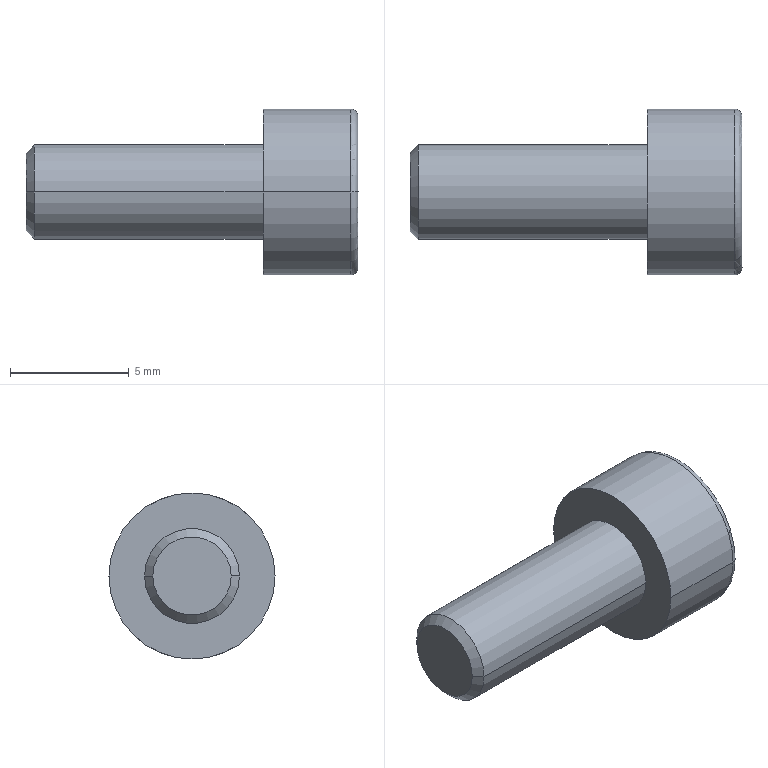Part | STEP file | 4-20.sldasm-Part-7 | 1 solid | 18 faces | box 14 x 7 x 7 mm | volume 262.874 mm3 | plane 10 | cylinder 4 | cone 2 | torus 2 | commonest cylinder face diameters 4 x2 7 x2
STEP:
#1=CARTESIAN_POINT('',(255.,438.35,193.));
#2=VERTEX_POINT('',#1);
#3=CARTESIAN_POINT('',(255.,441.651,193.));
#4=VERTEX_POINT('',#3);
#5=CARTESIAN_POINT('',(255.,440.,193.));
#6=DIRECTION('',(1.,0.000000295,0.));
#7=DIRECTION('',(-0.000000295,1.,-0.000000295));
#8=AXIS2_PLACEMENT_3D('',#5,#6,#7);
#9=CIRCLE('',#8,1.65);
#10=EDGE_CURVE('',#2,#4,#9,.T.);
#11=ORIENTED_EDGE('',*,*,#10,.T.);
#12=CARTESIAN_POINT('',(255.349,442.,193.));
#13=VERTEX_POINT('',#12);
#14=CARTESIAN_POINT('',(255.349,442.,193.));
#15=DIRECTION('',(0.7071,0.7071,-0.000000209));
#16=VECTOR('',#15,1000.);
#17=LINE('',#14,#16);
#18=EDGE_CURVE('',#4,#13,#17,.T.);
#19=ORIENTED_EDGE('',*,*,#18,.T.);
#20=CARTESIAN_POINT('',(255.349,438.,193.));
#21=VERTEX_POINT('',#20);
#22=CARTESIAN_POINT('',(255.349,440.,193.));
#23=DIRECTION('',(1.,0.000000295,0.));
#24=DIRECTION('',(-0.000000295,1.,-0.000000295));
#25=AXIS2_PLACEMENT_3D('',#22,#23,#24);
#26=CIRCLE('',#25,2.);
#27=EDGE_CURVE('',#21,#13,#26,.T.);
#28=ORIENTED_EDGE('',*,*,#27,.F.);
#29=CARTESIAN_POINT('',(255.349,438.,193.));
#30=DIRECTION('',(0.7071,-0.7071,0.000000209));
#31=VECTOR('',#30,1000.);
#32=LINE('',#29,#31);
#33=EDGE_CURVE('',#2,#21,#32,.T.);
#34=ORIENTED_EDGE('',*,*,#33,.F.);
#35=EDGE_LOOP('',(#11,#19,#28,#34));
#36=FACE_OUTER_BOUND('',#35,.T.);
#37=CARTESIAN_POINT('',(255.349,440.,193.));
#38=DIRECTION('',(1.,0.000000295,0.));
#39=DIRECTION('',(0.000000295,-1.,0.000000295));
#40=AXIS2_PLACEMENT_3D('',#37,#38,#39);
#41=CONICAL_SURFACE('',#40,2.,0.7854);
#42=ADVANCED_FACE('',(#36),#41,.T.);
#43=ORIENTED_EDGE('',*,*,#27,.T.);
#44=CARTESIAN_POINT('',(265.,442.,193.));
#45=VERTEX_POINT('',#44);
#46=CARTESIAN_POINT('',(270.675,442.,193.));
#47=DIRECTION('',(1.,0.000000295,0.));
#48=VECTOR('',#47,1000.);
#49=LINE('',#46,#48);
#50=EDGE_CURVE('',#13,#45,#49,.T.);
#51=ORIENTED_EDGE('',*,*,#50,.T.);
#52=CARTESIAN_POINT('',(265.,438.,193.));
#53=VERTEX_POINT('',#52);
#54=CARTESIAN_POINT('',(265.,440.,193.));
#55=DIRECTION('',(1.,0.000000295,0.));
#56=DIRECTION('',(-0.000000295,1.,-0.000000295));
#57=AXIS2_PLACEMENT_3D('',#54,#55,#56);
#58=CIRCLE('',#57,2.);
#59=EDGE_CURVE('',#53,#45,#58,.T.);
#60=ORIENTED_EDGE('',*,*,#59,.F.);
#61=CARTESIAN_POINT('',(270.675,438.,193.));
#62=DIRECTION('',(1.,0.000000295,0.));
#63=VECTOR('',#62,1000.);
#64=LINE('',#61,#63);
#65=EDGE_CURVE('',#21,#53,#64,.T.);
#66=ORIENTED_EDGE('',*,*,#65,.F.);
#67=EDGE_LOOP('',(#43,#51,#60,#66));
#68=FACE_OUTER_BOUND('',#67,.T.);
#69=CARTESIAN_POINT('',(270.675,440.,193.));
#70=DIRECTION('',(1.,0.000000295,0.));
#71=DIRECTION('',(0.000000295,-1.,0.000000295));
#72=AXIS2_PLACEMENT_3D('',#69,#70,#71);
#73=CYLINDRICAL_SURFACE('',#72,2.);
#74=ADVANCED_FACE('',(#68),#73,.T.);
#75=CARTESIAN_POINT('',(265.,436.5,193.));
#76=VERTEX_POINT('',#75);
#77=CARTESIAN_POINT('',(265.,443.5,193.));
#78=VERTEX_POINT('',#77);
#79=CARTESIAN_POINT('',(265.,440.,193.));
#80=DIRECTION('',(1.,0.000000295,0.));
#81=DIRECTION('',(-0.000000295,1.,-0.000000295));
#82=AXIS2_PLACEMENT_3D('',#79,#80,#81);
#83=CIRCLE('',#82,3.5);
#84=EDGE_CURVE('',#76,#78,#83,.T.);
#85=ORIENTED_EDGE('',*,*,#84,.T.);
#86=CARTESIAN_POINT('',(268.7,443.5,193.));
#87=VERTEX_POINT('',#86);
#88=CARTESIAN_POINT('',(270.675,443.5,193.));
#89=DIRECTION('',(1.,0.000000295,0.));
#90=VECTOR('',#89,1000.);
#91=LINE('',#88,#90);
#92=EDGE_CURVE('',#78,#87,#91,.T.);
#93=ORIENTED_EDGE('',*,*,#92,.T.);
#94=CARTESIAN_POINT('',(268.7,436.5,193.));
#95=VERTEX_POINT('',#94);
#96=CARTESIAN_POINT('',(268.7,440.,193.));
#97=DIRECTION('',(1.,0.000000295,0.));
#98=DIRECTION('',(-0.000000295,1.,-0.000000295));
#99=AXIS2_PLACEMENT_3D('',#96,#97,#98);
#100=CIRCLE('',#99,3.5);
#101=EDGE_CURVE('',#95,#87,#100,.T.);
#102=ORIENTED_EDGE('',*,*,#101,.F.);
#103=CARTESIAN_POINT('',(270.675,436.5,193.));
#104=DIRECTION('',(1.,0.000000295,0.));
#105=VECTOR('',#104,1000.);
#106=LINE('',#103,#105);
#107=EDGE_CURVE('',#76,#95,#106,.T.);
#108=ORIENTED_EDGE('',*,*,#107,.F.);
#109=EDGE_LOOP('',(#85,#93,#102,#108));
#110=FACE_OUTER_BOUND('',#109,.T.);
#111=CARTESIAN_POINT('',(270.675,440.,193.));
#112=DIRECTION('',(1.,0.000000295,0.));
#113=DIRECTION('',(0.000000295,-1.,0.000000295));
#114=AXIS2_PLACEMENT_3D('',#111,#112,#113);
#115=CYLINDRICAL_SURFACE('',#114,3.5);
#116=ADVANCED_FACE('',(#110),#115,.T.);
#117=ORIENTED_EDGE('',*,*,#101,.T.);
#118=CARTESIAN_POINT('',(269.,443.2,193.));
#119=VERTEX_POINT('',#118);
#120=CARTESIAN_POINT('',(268.7,443.2,193.));
#121=DIRECTION('',(0.,-0.000000295,-1.));
#122=DIRECTION('',(0.,1.,-0.000000295));
#123=AXIS2_PLACEMENT_3D('',#120,#121,#122);
#124=CIRCLE('',#123,0.3);
#125=EDGE_CURVE('',#87,#119,#124,.T.);
#126=ORIENTED_EDGE('',*,*,#125,.T.);
#127=CARTESIAN_POINT('',(269.,436.8,193.));
#128=VERTEX_POINT('',#127);
#129=CARTESIAN_POINT('',(269.,440.,193.));
#130=DIRECTION('',(1.,0.000000295,0.));
#131=DIRECTION('',(-0.000000295,1.,-0.000000295));
#132=AXIS2_PLACEMENT_3D('',#129,#130,#131);
#133=CIRCLE('',#132,3.2);
#134=EDGE_CURVE('',#128,#119,#133,.T.);
#135=ORIENTED_EDGE('',*,*,#134,.F.);
#136=CARTESIAN_POINT('',(268.7,436.8,193.));
#137=DIRECTION('',(0.,0.000000295,1.));
#138=DIRECTION('',(0.,-1.,0.000000295));
#139=AXIS2_PLACEMENT_3D('',#136,#137,#138);
#140=CIRCLE('',#139,0.3);
#141=EDGE_CURVE('',#95,#128,#140,.T.);
#142=ORIENTED_EDGE('',*,*,#141,.F.);
#143=EDGE_LOOP('',(#117,#126,#135,#142));
#144=FACE_OUTER_BOUND('',#143,.T.);
#145=CARTESIAN_POINT('',(268.7,440.,193.));
#146=DIRECTION('',(1.,0.000000295,0.));
#147=DIRECTION('',(0.000000295,-1.,0.000000295));
#148=AXIS2_PLACEMENT_3D('',#145,#146,#147);
#149=TOROIDAL_SURFACE('',#148,3.2,0.3);
#150=ADVANCED_FACE('',(#144),#149,.T.);
#151=CARTESIAN_POINT('',(269.,441.5,193.866));
#152=VERTEX_POINT('',#151);
#153=CARTESIAN_POINT('',(269.,440.,194.732));
#154=VERTEX_POINT('',#153);
#155=CARTESIAN_POINT('',(269.,441.5,193.866));
#156=DIRECTION('',(0.000000256,-0.866,0.5));
#157=VECTOR('',#156,1000.);
#158=LINE('',#155,#157);
#159=EDGE_CURVE('',#152,#154,#158,.T.);
#160=ORIENTED_EDGE('',*,*,#159,.F.);
#161=CARTESIAN_POINT('',(269.,441.5,192.134));
#162=VERTEX_POINT('',#161);
#163=CARTESIAN_POINT('',(269.,441.5,192.134));
#164=DIRECTION('',(0.,0.000000295,1.));
#165=VECTOR('',#164,1000.);
#166=LINE('',#163,#165);
#167=EDGE_CURVE('',#162,#152,#166,.T.);
#168=ORIENTED_EDGE('',*,*,#167,.F.);
#169=CARTESIAN_POINT('',(269.,440.,191.268));
#170=VERTEX_POINT('',#169);
#171=CARTESIAN_POINT('',(269.,440.,191.268));
#172=DIRECTION('',(-0.000000256,0.866,0.5));
#173=VECTOR('',#172,1000.);
#174=LINE('',#171,#173);
#175=EDGE_CURVE('',#170,#162,#174,.T.);
#176=ORIENTED_EDGE('',*,*,#175,.F.);
#177=CARTESIAN_POINT('',(269.,438.5,192.134));
#178=VERTEX_POINT('',#177);
#179=CARTESIAN_POINT('',(269.,438.5,192.134));
#180=DIRECTION('',(-0.000000256,0.866,-0.5));
#181=VECTOR('',#180,1000.);
#182=LINE('',#179,#181);
#183=EDGE_CURVE('',#178,#170,#182,.T.);
#184=ORIENTED_EDGE('',*,*,#183,.F.);
#185=CARTESIAN_POINT('',(269.,438.5,193.866));
#186=VERTEX_POINT('',#185);
#187=CARTESIAN_POINT('',(269.,438.5,193.866));
#188=DIRECTION('',(0.,-0.000000295,-1.));
#189=VECTOR('',#188,1000.);
#190=LINE('',#187,#189);
#191=EDGE_CURVE('',#186,#178,#190,.T.);
#192=ORIENTED_EDGE('',*,*,#191,.F.);
#193=CARTESIAN_POINT('',(269.,440.,194.732));
#194=DIRECTION('',(0.000000256,-0.866,-0.5));
#195=VECTOR('',#194,1000.);
#196=LINE('',#193,#195);
#197=EDGE_CURVE('',#154,#186,#196,.T.);
#198=ORIENTED_EDGE('',*,*,#197,.F.);
#199=EDGE_LOOP('',(#160,#168,#176,#184,#192,#198));
#200=FACE_BOUND('',#199,.T.);
#201=ORIENTED_EDGE('',*,*,#134,.T.);
#202=CARTESIAN_POINT('',(269.,440.,193.));
#203=DIRECTION('',(1.,0.000000295,0.));
#204=DIRECTION('',(-0.000000295,1.,-0.000000295));
#205=AXIS2_PLACEMENT_3D('',#202,#203,#204);
#206=CIRCLE('',#205,3.2);
#207=EDGE_CURVE('',#119,#128,#206,.T.);
#208=ORIENTED_EDGE('',*,*,#207,.T.);
#209=EDGE_LOOP('',(#201,#208));
#210=FACE_OUTER_BOUND('',#209,.T.);
#211=CARTESIAN_POINT('',(269.,440.,193.));
#212=DIRECTION('',(1.,0.000000295,0.));
#213=DIRECTION('',(0.000000295,-1.,0.000000295));
#214=AXIS2_PLACEMENT_3D('',#211,#212,#213);
#215=PLANE('',#214);
#216=ADVANCED_FACE('',(#200,#210),#215,.T.);
#217=ORIENTED_EDGE('',*,*,#125,.F.);
#218=CARTESIAN_POINT('',(268.7,440.,193.));
#219=DIRECTION('',(1.,0.000000295,0.));
#220=DIRECTION('',(-0.000000295,1.,-0.000000295));
#221=AXIS2_PLACEMENT_3D('',#218,#219,#220);
#222=CIRCLE('',#221,3.5);
#223=EDGE_CURVE('',#87,#95,#222,.T.);
#224=ORIENTED_EDGE('',*,*,#223,.T.);
#225=ORIENTED_EDGE('',*,*,#141,.T.);
#226=ORIENTED_EDGE('',*,*,#207,.F.);
#227=EDGE_LOOP('',(#217,#224,#225,#226));
#228=FACE_OUTER_BOUND('',#227,.T.);
#229=CARTESIAN_POINT('',(268.7,440.,193.));
#230=DIRECTION('',(1.,0.000000295,0.));
#231=DIRECTION('',(0.000000295,-1.,0.000000295));
#232=AXIS2_PLACEMENT_3D('',#229,#230,#231);
#233=TOROIDAL_SURFACE('',#232,3.2,0.3);
#234=ADVANCED_FACE('',(#228),#233,.T.);
#235=ORIENTED_EDGE('',*,*,#92,.F.);
#236=CARTESIAN_POINT('',(265.,440.,193.));
#237=DIRECTION('',(1.,0.000000295,0.));
#238=DIRECTION('',(-0.000000295,1.,-0.000000295));
#239=AXIS2_PLACEMENT_3D('',#236,#237,#238);
#240=CIRCLE('',#239,3.5);
#241=EDGE_CURVE('',#78,#76,#240,.T.);
#242=ORIENTED_EDGE('',*,*,#241,.T.);
#243=ORIENTED_EDGE('',*,*,#107,.T.);
#244=ORIENTED_EDGE('',*,*,#223,.F.);
#245=EDGE_LOOP('',(#235,#242,#243,#244));
#246=FACE_OUTER_BOUND('',#245,.T.);
#247=CARTESIAN_POINT('',(270.675,440.,193.));
#248=DIRECTION('',(1.,0.000000295,0.));
#249=DIRECTION('',(0.000000295,-1.,0.000000295));
#250=AXIS2_PLACEMENT_3D('',#247,#248,#249);
#251=CYLINDRICAL_SURFACE('',#250,3.5);
#252=ADVANCED_FACE('',(#246),#251,.T.);
#253=ORIENTED_EDGE('',*,*,#59,.T.);
#254=CARTESIAN_POINT('',(265.,440.,193.));
#255=DIRECTION('',(1.,0.000000295,0.));
#256=DIRECTION('',(-0.000000295,1.,-0.000000295));
#257=AXIS2_PLACEMENT_3D('',#254,#255,#256);
#258=CIRCLE('',#257,2.);
#259=EDGE_CURVE('',#45,#53,#258,.T.);
#260=ORIENTED_EDGE('',*,*,#259,.T.);
#261=EDGE_LOOP('',(#253,#260));
#262=FACE_BOUND('',#261,.T.);
#263=ORIENTED_EDGE('',*,*,#84,.F.);
#264=ORIENTED_EDGE('',*,*,#241,.F.);
#265=EDGE_LOOP('',(#263,#264));
#266=FACE_OUTER_BOUND('',#265,.T.);
#267=CARTESIAN_POINT('',(265.,440.,196.5));
#268=DIRECTION('',(-1.,-0.000000295,0.));
#269=DIRECTION('',(-0.000000295,1.,-0.000000295));
#270=AXIS2_PLACEMENT_3D('',#267,#268,#269);
#271=PLANE('',#270);
#272=ADVANCED_FACE('',(#262,#266),#271,.T.);
#273=ORIENTED_EDGE('',*,*,#50,.F.);
#274=CARTESIAN_POINT('',(255.349,440.,193.));
#275=DIRECTION('',(1.,0.000000295,0.));
#276=DIRECTION('',(-0.000000295,1.,-0.000000295));
#277=AXIS2_PLACEMENT_3D('',#274,#275,#276);
#278=CIRCLE('',#277,2.);
#279=EDGE_CURVE('',#13,#21,#278,.T.);
#280=ORIENTED_EDGE('',*,*,#279,.T.);
#281=ORIENTED_EDGE('',*,*,#65,.T.);
#282=ORIENTED_EDGE('',*,*,#259,.F.);
#283=EDGE_LOOP('',(#273,#280,#281,#282));
#284=FACE_OUTER_BOUND('',#283,.T.);
#285=CARTESIAN_POINT('',(270.675,440.,193.));
#286=DIRECTION('',(1.,0.000000295,0.));
#287=DIRECTION('',(0.000000295,-1.,0.000000295));
#288=AXIS2_PLACEMENT_3D('',#285,#286,#287);
#289=CYLINDRICAL_SURFACE('',#288,2.);
#290=ADVANCED_FACE('',(#284),#289,.T.);
#291=ORIENTED_EDGE('',*,*,#18,.F.);
#292=CARTESIAN_POINT('',(255.,440.,193.));
#293=DIRECTION('',(1.,0.000000295,0.));
#294=DIRECTION('',(-0.000000295,1.,-0.000000295));
#295=AXIS2_PLACEMENT_3D('',#292,#293,#294);
#296=CIRCLE('',#295,1.65);
#297=EDGE_CURVE('',#4,#2,#296,.T.);
#298=ORIENTED_EDGE('',*,*,#297,.T.);
#299=ORIENTED_EDGE('',*,*,#33,.T.);
#300=ORIENTED_EDGE('',*,*,#279,.F.);
#301=EDGE_LOOP('',(#291,#298,#299,#300));
#302=FACE_OUTER_BOUND('',#301,.T.);
#303=CARTESIAN_POINT('',(255.349,440.,193.));
#304=DIRECTION('',(1.,0.000000295,0.));
#305=DIRECTION('',(0.000000295,-1.,0.000000295));
#306=AXIS2_PLACEMENT_3D('',#303,#304,#305);
#307=CONICAL_SURFACE('',#306,2.,0.7854);
#308=ADVANCED_FACE('',(#302),#307,.T.);
#309=ORIENTED_EDGE('',*,*,#10,.F.);
#310=ORIENTED_EDGE('',*,*,#297,.F.);
#311=EDGE_LOOP('',(#309,#310));
#312=FACE_OUTER_BOUND('',#311,.T.);
#313=CARTESIAN_POINT('',(255.,440.,194.65));
#314=DIRECTION('',(-1.,-0.000000295,0.));
#315=DIRECTION('',(-0.000000295,1.,-0.000000295));
#316=AXIS2_PLACEMENT_3D('',#313,#314,#315);
#317=PLANE('',#316);
#318=ADVANCED_FACE('',(#312),#317,.T.);
#319=ORIENTED_EDGE('',*,*,#159,.T.);
#320=CARTESIAN_POINT('',(267.,440.,194.732));
#321=VERTEX_POINT('',#320);
#322=CARTESIAN_POINT('',(267.,440.,194.732));
#323=DIRECTION('',(1.,0.000000295,0.));
#324=VECTOR('',#323,1000.);
#325=LINE('',#322,#324);
#326=EDGE_CURVE('',#321,#154,#325,.T.);
#327=ORIENTED_EDGE('',*,*,#326,.F.);
#328=CARTESIAN_POINT('',(267.,441.5,193.866));
#329=VERTEX_POINT('',#328);
#330=CARTESIAN_POINT('',(267.,441.5,193.866));
#331=DIRECTION('',(0.000000256,-0.866,0.5));
#332=VECTOR('',#331,1000.);
#333=LINE('',#330,#332);
#334=EDGE_CURVE('',#329,#321,#333,.T.);
#335=ORIENTED_EDGE('',*,*,#334,.F.);
#336=CARTESIAN_POINT('',(267.,441.5,193.866));
#337=DIRECTION('',(1.,0.000000295,0.));
#338=VECTOR('',#337,1000.);
#339=LINE('',#336,#338);
#340=EDGE_CURVE('',#329,#152,#339,.T.);
#341=ORIENTED_EDGE('',*,*,#340,.T.);
#342=EDGE_LOOP('',(#319,#327,#335,#341));
#343=FACE_OUTER_BOUND('',#342,.T.);
#344=CARTESIAN_POINT('',(267.,441.5,193.866));
#345=DIRECTION('',(-0.000000148,0.5,0.866));
#346=DIRECTION('',(-0.000000256,0.866,-0.5));
#347=AXIS2_PLACEMENT_3D('',#344,#345,#346);
#348=PLANE('',#347);
#349=ADVANCED_FACE('',(#343),#348,.F.);
#350=ORIENTED_EDGE('',*,*,#167,.T.);
#351=ORIENTED_EDGE('',*,*,#340,.F.);
#352=CARTESIAN_POINT('',(267.,441.5,192.134));
#353=VERTEX_POINT('',#352);
#354=CARTESIAN_POINT('',(267.,441.5,192.134));
#355=DIRECTION('',(0.,0.000000295,1.));
#356=VECTOR('',#355,1000.);
#357=LINE('',#354,#356);
#358=EDGE_CURVE('',#353,#329,#357,.T.);
#359=ORIENTED_EDGE('',*,*,#358,.F.);
#360=CARTESIAN_POINT('',(267.,441.5,192.134));
#361=DIRECTION('',(1.,0.000000295,0.));
#362=VECTOR('',#361,1000.);
#363=LINE('',#360,#362);
#364=EDGE_CURVE('',#353,#162,#363,.T.);
#365=ORIENTED_EDGE('',*,*,#364,.T.);
#366=EDGE_LOOP('',(#350,#351,#359,#365));
#367=FACE_OUTER_BOUND('',#366,.T.);
#368=CARTESIAN_POINT('',(267.,441.5,192.134));
#369=DIRECTION('',(-0.000000295,1.,-0.000000295));
#370=DIRECTION('',(1.,0.000000295,0.));
#371=AXIS2_PLACEMENT_3D('',#368,#369,#370);
#372=PLANE('',#371);
#373=ADVANCED_FACE('',(#367),#372,.F.);
#374=ORIENTED_EDGE('',*,*,#175,.T.);
#375=ORIENTED_EDGE('',*,*,#364,.F.);
#376=CARTESIAN_POINT('',(267.,440.,191.268));
#377=VERTEX_POINT('',#376);
#378=CARTESIAN_POINT('',(267.,440.,191.268));
#379=DIRECTION('',(-0.000000256,0.866,0.5));
#380=VECTOR('',#379,1000.);
#381=LINE('',#378,#380);
#382=EDGE_CURVE('',#377,#353,#381,.T.);
#383=ORIENTED_EDGE('',*,*,#382,.F.);
#384=CARTESIAN_POINT('',(267.,440.,191.268));
#385=DIRECTION('',(1.,0.000000295,0.));
#386=VECTOR('',#385,1000.);
#387=LINE('',#384,#386);
#388=EDGE_CURVE('',#377,#170,#387,.T.);
#389=ORIENTED_EDGE('',*,*,#388,.T.);
#390=EDGE_LOOP('',(#374,#375,#383,#389));
#391=FACE_OUTER_BOUND('',#390,.T.);
#392=CARTESIAN_POINT('',(267.,440.,191.268));
#393=DIRECTION('',(-0.000000148,0.5,-0.866));
#394=DIRECTION('',(0.000000256,-0.866,-0.5));
#395=AXIS2_PLACEMENT_3D('',#392,#393,#394);
#396=PLANE('',#395);
#397=ADVANCED_FACE('',(#391),#396,.F.);
#398=ORIENTED_EDGE('',*,*,#183,.T.);
#399=ORIENTED_EDGE('',*,*,#388,.F.);
#400=CARTESIAN_POINT('',(267.,438.5,192.134));
#401=VERTEX_POINT('',#400);
#402=CARTESIAN_POINT('',(267.,438.5,192.134));
#403=DIRECTION('',(-0.000000256,0.866,-0.5));
#404=VECTOR('',#403,1000.);
#405=LINE('',#402,#404);
#406=EDGE_CURVE('',#401,#377,#405,.T.);
#407=ORIENTED_EDGE('',*,*,#406,.F.);
#408=CARTESIAN_POINT('',(267.,438.5,192.134));
#409=DIRECTION('',(1.,0.000000295,0.));
#410=VECTOR('',#409,1000.);
#411=LINE('',#408,#410);
#412=EDGE_CURVE('',#401,#178,#411,.T.);
#413=ORIENTED_EDGE('',*,*,#412,.T.);
#414=EDGE_LOOP('',(#398,#399,#407,#413));
#415=FACE_OUTER_BOUND('',#414,.T.);
#416=CARTESIAN_POINT('',(267.,438.5,192.134));
#417=DIRECTION('',(0.000000148,-0.5,-0.866));
#418=DIRECTION('',(0.000000256,-0.866,0.5));
#419=AXIS2_PLACEMENT_3D('',#416,#417,#418);
#420=PLANE('',#419);
#421=ADVANCED_FACE('',(#415),#420,.F.);
#422=ORIENTED_EDGE('',*,*,#191,.T.);
#423=ORIENTED_EDGE('',*,*,#412,.F.);
#424=CARTESIAN_POINT('',(267.,438.5,193.866));
#425=VERTEX_POINT('',#424);
#426=CARTESIAN_POINT('',(267.,438.5,193.866));
#427=DIRECTION('',(0.,-0.000000295,-1.));
#428=VECTOR('',#427,1000.);
#429=LINE('',#426,#428);
#430=EDGE_CURVE('',#425,#401,#429,.T.);
#431=ORIENTED_EDGE('',*,*,#430,.F.);
#432=CARTESIAN_POINT('',(267.,438.5,193.866));
#433=DIRECTION('',(1.,0.000000295,0.));
#434=VECTOR('',#433,1000.);
#435=LINE('',#432,#434);
#436=EDGE_CURVE('',#425,#186,#435,.T.);
#437=ORIENTED_EDGE('',*,*,#436,.T.);
#438=EDGE_LOOP('',(#422,#423,#431,#437));
#439=FACE_OUTER_BOUND('',#438,.T.);
#440=CARTESIAN_POINT('',(267.,438.5,193.866));
#441=DIRECTION('',(0.000000295,-1.,0.000000295));
#442=DIRECTION('',(-1.,-0.000000295,0.));
#443=AXIS2_PLACEMENT_3D('',#440,#441,#442);
#444=PLANE('',#443);
#445=ADVANCED_FACE('',(#439),#444,.F.);
#446=ORIENTED_EDGE('',*,*,#197,.T.);
#447=ORIENTED_EDGE('',*,*,#436,.F.);
#448=CARTESIAN_POINT('',(267.,440.,194.732));
#449=DIRECTION('',(0.000000256,-0.866,-0.5));
#450=VECTOR('',#449,1000.);
#451=LINE('',#448,#450);
#452=EDGE_CURVE('',#321,#425,#451,.T.);
#453=ORIENTED_EDGE('',*,*,#452,.F.);
#454=ORIENTED_EDGE('',*,*,#326,.T.);
#455=EDGE_LOOP('',(#446,#447,#453,#454));
#456=FACE_OUTER_BOUND('',#455,.T.);
#457=CARTESIAN_POINT('',(267.,440.,194.732));
#458=DIRECTION('',(0.000000148,-0.5,0.866));
#459=DIRECTION('',(-0.000000256,0.866,0.5));
#460=AXIS2_PLACEMENT_3D('',#457,#458,#459);
#461=PLANE('',#460);
#462=ADVANCED_FACE('',(#456),#461,.F.);
#463=ORIENTED_EDGE('',*,*,#334,.T.);
#464=ORIENTED_EDGE('',*,*,#452,.T.);
#465=ORIENTED_EDGE('',*,*,#430,.T.);
#466=ORIENTED_EDGE('',*,*,#406,.T.);
#467=ORIENTED_EDGE('',*,*,#382,.T.);
#468=ORIENTED_EDGE('',*,*,#358,.T.);
#469=EDGE_LOOP('',(#463,#464,#465,#466,#467,#468));
#470=FACE_OUTER_BOUND('',#469,.T.);
#471=CARTESIAN_POINT('',(267.,441.5,193.866));
#472=DIRECTION('',(-1.,-0.000000295,0.));
#473=DIRECTION('',(-0.000000295,1.,-0.000000295));
#474=AXIS2_PLACEMENT_3D('',#471,#472,#473);
#475=PLANE('',#474);
#476=ADVANCED_FACE('',(#470),#475,.F.);
#477=CLOSED_SHELL('',(#42,#74,#116,#150,#216,#234,#252,#272,#290,#308,#318,#349,#373,#397,#421,#445,#462,#476));
#478=MANIFOLD_SOLID_BREP('',#477);
#479=CARTESIAN_POINT('',(0.,0.,0.));
#480=DIRECTION('',(0.,0.,1.));
#481=DIRECTION('',(1.,0.,0.));
#482=AXIS2_PLACEMENT_3D('',#479,#480,#481);
#483=(LENGTH_UNIT()NAMED_UNIT(*)SI_UNIT(.MILLI.,.METRE.));
#484=UNCERTAINTY_MEASURE_WITH_UNIT(LENGTH_MEASURE(0.00001),#483,'','');
#485=(NAMED_UNIT(*)PLANE_ANGLE_UNIT()SI_UNIT($,.RADIAN.));
#486=(NAMED_UNIT(*)SI_UNIT($,.STERADIAN.)SOLID_ANGLE_UNIT());
#487=(GEOMETRIC_REPRESENTATION_CONTEXT(3)GLOBAL_UNCERTAINTY_ASSIGNED_CONTEXT((#484))GLOBAL_UNIT_ASSIGNED_CONTEXT((#483,#485,#486))REPRESENTATION_CONTEXT('',''));
#488=ADVANCED_BREP_SHAPE_REPRESENTATION('',(#478,#482),#487);